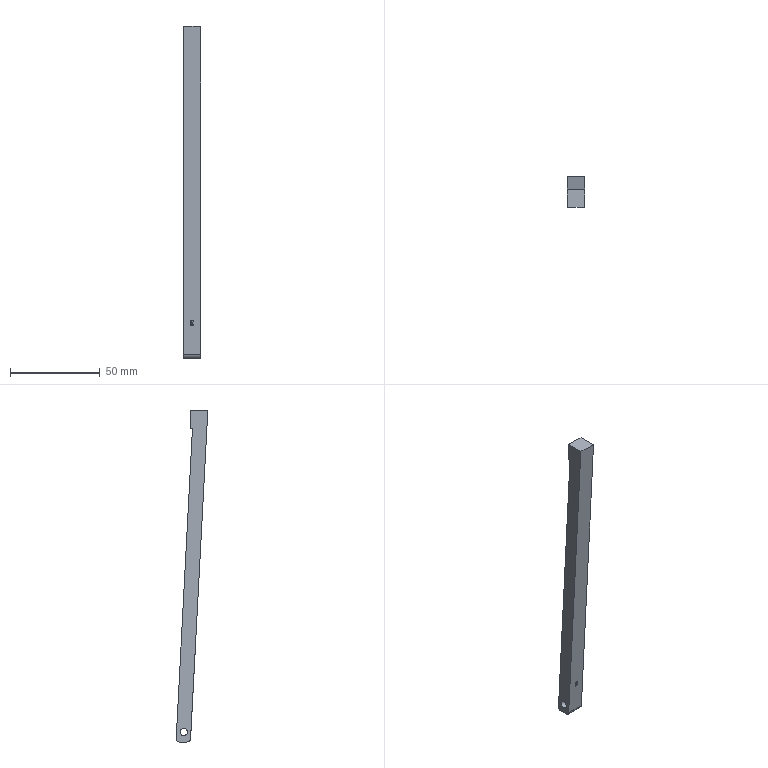Part | STEP file | solid 26 | 1 solid | 34 faces | box 10 x 17.589 x 184.804 mm | volume 14786 mm3 | plane 25 | cylinder 5 | other 4 | commonest cylinder face diameters 4 x3 1.005 x1 6922 x1